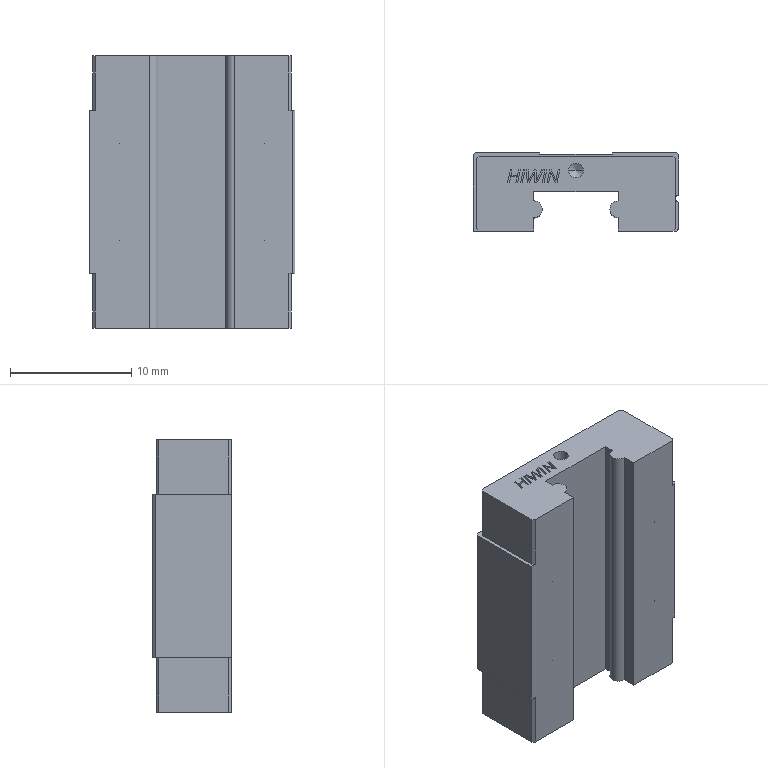Part | STEP file | MGN7C-slider block | 1 solid | 187 faces | box 17 x 6.5 x 22.5 mm | volume 1844 mm3 | plane 120 | spline 38 | cylinder 17 | cone 12 | commonest cylinder face diameters 1.6 x8 1.2 x4 1.4 x3 0.6 x2